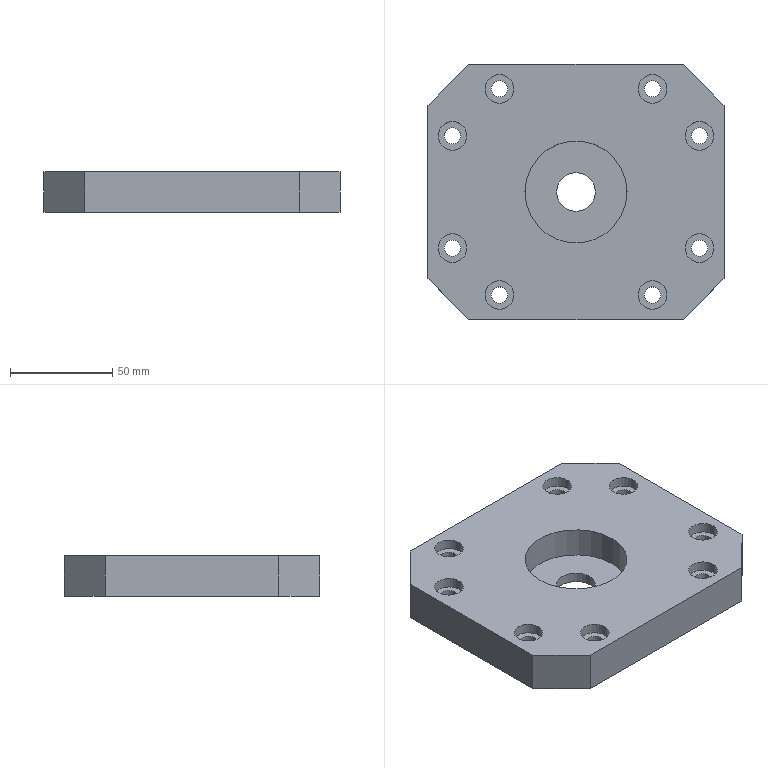Part | SolidWorks | features ICE 6, Chamfer 1, Extrusion 1 | 1 solid | 55 faces | box 145 x 125 x 20 mm | volume 303441 mm3 | cylinder 36 | plane 19 | commonest cylinder face diameters 8 x16 14 x16 19 x2 50 x2